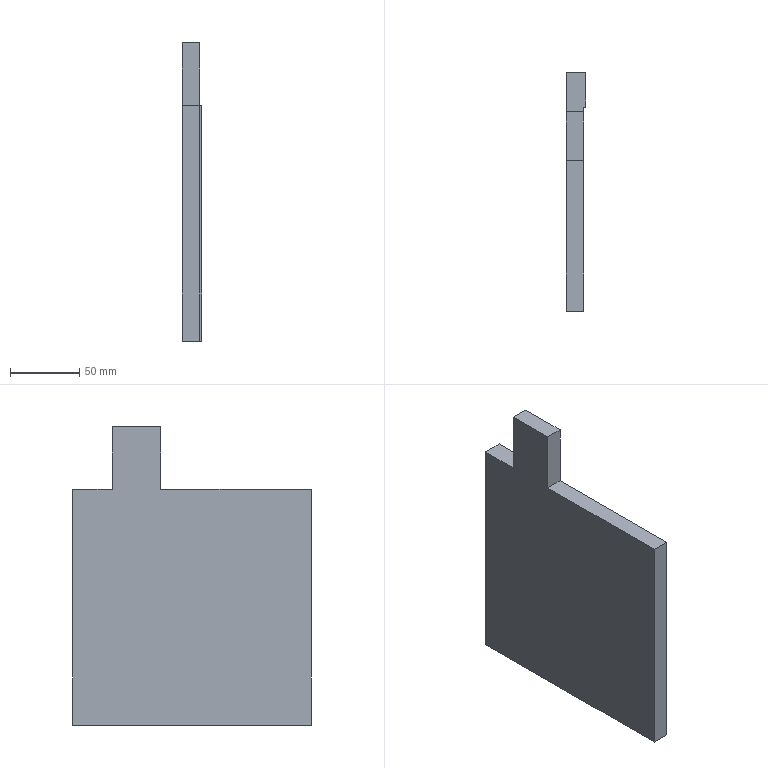Part | SolidWorks | features ICE 2, 3DProfileFeature 1, Extrusion 1, HoleWzd 1 | 1 solid | 12 faces | box 14 x 172 x 215 mm | volume 391562 mm3 | plane 12
STEP:
#1=CARTESIAN_POINT('',(12.5,0.,85.));
#2=VERTEX_POINT('',#1);
#3=CARTESIAN_POINT('',(12.5,108.5,85.));
#4=VERTEX_POINT('',#3);
#5=CARTESIAN_POINT('',(12.5,147.,85.));
#6=DIRECTION('',(0.,1.,0.));
#7=VECTOR('',#6,1000.);
#8=LINE('',#5,#7);
#9=EDGE_CURVE('',#2,#4,#8,.T.);
#10=ORIENTED_EDGE('',*,*,#9,.T.);
#11=CARTESIAN_POINT('',(0.,108.5,85.));
#12=VERTEX_POINT('',#11);
#13=CARTESIAN_POINT('',(12.5,108.5,85.));
#14=DIRECTION('',(-1.,0.,0.));
#15=VECTOR('',#14,1000.);
#16=LINE('',#13,#15);
#17=EDGE_CURVE('',#4,#12,#16,.T.);
#18=ORIENTED_EDGE('',*,*,#17,.T.);
#19=CARTESIAN_POINT('',(0.,0.,85.));
#20=VERTEX_POINT('',#19);
#21=CARTESIAN_POINT('',(0.,0.,85.));
#22=DIRECTION('',(0.,-1.,0.));
#23=VECTOR('',#22,1000.);
#24=LINE('',#21,#23);
#25=EDGE_CURVE('',#12,#20,#24,.T.);
#26=ORIENTED_EDGE('',*,*,#25,.T.);
#27=CARTESIAN_POINT('',(12.5,0.,85.));
#28=DIRECTION('',(1.,0.,0.));
#29=VECTOR('',#28,1000.);
#30=LINE('',#27,#29);
#31=EDGE_CURVE('',#20,#2,#30,.T.);
#32=ORIENTED_EDGE('',*,*,#31,.T.);
#33=EDGE_LOOP('',(#10,#18,#26,#32));
#34=FACE_OUTER_BOUND('',#33,.T.);
#35=CARTESIAN_POINT('',(0.,0.,85.));
#36=DIRECTION('',(0.,0.,-1.));
#37=DIRECTION('',(-1.,0.,0.));
#38=AXIS2_PLACEMENT_3D('',#35,#36,#37);
#39=PLANE('',#38);
#40=ADVANCED_FACE('',(#34),#39,.F.);
#41=CARTESIAN_POINT('',(0.,0.,-85.));
#42=VERTEX_POINT('',#41);
#43=CARTESIAN_POINT('',(12.5,0.,-85.));
#44=VERTEX_POINT('',#43);
#45=CARTESIAN_POINT('',(12.5,0.,-85.));
#46=DIRECTION('',(1.,0.,0.));
#47=VECTOR('',#46,1000.);
#48=LINE('',#45,#47);
#49=EDGE_CURVE('',#42,#44,#48,.T.);
#50=ORIENTED_EDGE('',*,*,#49,.T.);
#51=CARTESIAN_POINT('',(12.5,0.,85.));
#52=DIRECTION('',(0.,0.,-1.));
#53=VECTOR('',#52,1000.);
#54=LINE('',#51,#53);
#55=EDGE_CURVE('',#2,#44,#54,.T.);
#56=ORIENTED_EDGE('',*,*,#55,.F.);
#57=ORIENTED_EDGE('',*,*,#31,.F.);
#58=CARTESIAN_POINT('',(0.,0.,85.));
#59=DIRECTION('',(0.,0.,-1.));
#60=VECTOR('',#59,1000.);
#61=LINE('',#58,#60);
#62=EDGE_CURVE('',#20,#42,#61,.T.);
#63=ORIENTED_EDGE('',*,*,#62,.T.);
#64=EDGE_LOOP('',(#50,#56,#57,#63));
#65=FACE_OUTER_BOUND('',#64,.T.);
#66=CARTESIAN_POINT('',(12.5,0.,85.));
#67=DIRECTION('',(0.,1.,0.));
#68=DIRECTION('',(-1.,0.,0.));
#69=AXIS2_PLACEMENT_3D('',#66,#67,#68);
#70=PLANE('',#69);
#71=ADVANCED_FACE('',(#65),#70,.F.);
#72=CARTESIAN_POINT('',(12.5,147.,-85.));
#73=VERTEX_POINT('',#72);
#74=CARTESIAN_POINT('',(12.5,147.,-85.));
#75=DIRECTION('',(0.,1.,0.));
#76=VECTOR('',#75,1000.);
#77=LINE('',#74,#76);
#78=EDGE_CURVE('',#44,#73,#77,.T.);
#79=ORIENTED_EDGE('',*,*,#78,.T.);
#80=CARTESIAN_POINT('',(12.5,147.,85.));
#81=VERTEX_POINT('',#80);
#82=CARTESIAN_POINT('',(12.5,147.,85.));
#83=DIRECTION('',(0.,0.,-1.));
#84=VECTOR('',#83,1000.);
#85=LINE('',#82,#84);
#86=EDGE_CURVE('',#81,#73,#85,.T.);
#87=ORIENTED_EDGE('',*,*,#86,.F.);
#88=CARTESIAN_POINT('',(12.5,143.5,85.));
#89=VERTEX_POINT('',#88);
#90=CARTESIAN_POINT('',(12.5,147.,85.));
#91=DIRECTION('',(0.,1.,0.));
#92=VECTOR('',#91,1000.);
#93=LINE('',#90,#92);
#94=EDGE_CURVE('',#89,#81,#93,.T.);
#95=ORIENTED_EDGE('',*,*,#94,.F.);
#96=CARTESIAN_POINT('',(12.5,143.5,130.));
#97=VERTEX_POINT('',#96);
#98=CARTESIAN_POINT('',(12.5,143.5,130.));
#99=DIRECTION('',(0.,0.,-1.));
#100=VECTOR('',#99,1000.);
#101=LINE('',#98,#100);
#102=EDGE_CURVE('',#97,#89,#101,.T.);
#103=ORIENTED_EDGE('',*,*,#102,.F.);
#104=CARTESIAN_POINT('',(12.5,108.5,130.));
#105=VERTEX_POINT('',#104);
#106=CARTESIAN_POINT('',(12.5,143.5,130.));
#107=DIRECTION('',(0.,-1.,0.));
#108=VECTOR('',#107,1000.);
#109=LINE('',#106,#108);
#110=EDGE_CURVE('',#97,#105,#109,.T.);
#111=ORIENTED_EDGE('',*,*,#110,.T.);
#112=CARTESIAN_POINT('',(12.5,108.5,130.));
#113=DIRECTION('',(0.,0.,-1.));
#114=VECTOR('',#113,1000.);
#115=LINE('',#112,#114);
#116=EDGE_CURVE('',#105,#4,#115,.T.);
#117=ORIENTED_EDGE('',*,*,#116,.T.);
#118=ORIENTED_EDGE('',*,*,#9,.F.);
#119=ORIENTED_EDGE('',*,*,#55,.T.);
#120=EDGE_LOOP('',(#79,#87,#95,#103,#111,#117,#118,#119));
#121=FACE_OUTER_BOUND('',#120,.T.);
#122=CARTESIAN_POINT('',(12.5,147.,85.));
#123=DIRECTION('',(-1.,0.,0.));
#124=DIRECTION('',(0.,-1.,0.));
#125=AXIS2_PLACEMENT_3D('',#122,#123,#124);
#126=PLANE('',#125);
#127=ADVANCED_FACE('',(#121),#126,.F.);
#128=CARTESIAN_POINT('',(14.,147.,-85.));
#129=VERTEX_POINT('',#128);
#130=CARTESIAN_POINT('',(14.,147.,-85.));
#131=DIRECTION('',(1.,0.,0.));
#132=VECTOR('',#131,1000.);
#133=LINE('',#130,#132);
#134=EDGE_CURVE('',#73,#129,#133,.T.);
#135=ORIENTED_EDGE('',*,*,#134,.T.);
#136=CARTESIAN_POINT('',(14.,147.,85.));
#137=VERTEX_POINT('',#136);
#138=CARTESIAN_POINT('',(14.,147.,85.));
#139=DIRECTION('',(0.,0.,-1.));
#140=VECTOR('',#139,1000.);
#141=LINE('',#138,#140);
#142=EDGE_CURVE('',#137,#129,#141,.T.);
#143=ORIENTED_EDGE('',*,*,#142,.F.);
#144=CARTESIAN_POINT('',(14.,147.,85.));
#145=DIRECTION('',(1.,0.,0.));
#146=VECTOR('',#145,1000.);
#147=LINE('',#144,#146);
#148=EDGE_CURVE('',#81,#137,#147,.T.);
#149=ORIENTED_EDGE('',*,*,#148,.F.);
#150=ORIENTED_EDGE('',*,*,#86,.T.);
#151=EDGE_LOOP('',(#135,#143,#149,#150));
#152=FACE_OUTER_BOUND('',#151,.T.);
#153=CARTESIAN_POINT('',(14.,147.,85.));
#154=DIRECTION('',(0.,1.,0.));
#155=DIRECTION('',(0.,0.,1.));
#156=AXIS2_PLACEMENT_3D('',#153,#154,#155);
#157=PLANE('',#156);
#158=ADVANCED_FACE('',(#152),#157,.F.);
#159=CARTESIAN_POINT('',(14.,172.,-85.));
#160=VERTEX_POINT('',#159);
#161=CARTESIAN_POINT('',(14.,172.,-85.));
#162=DIRECTION('',(0.,1.,0.));
#163=VECTOR('',#162,1000.);
#164=LINE('',#161,#163);
#165=EDGE_CURVE('',#129,#160,#164,.T.);
#166=ORIENTED_EDGE('',*,*,#165,.T.);
#167=CARTESIAN_POINT('',(14.,172.,85.));
#168=VERTEX_POINT('',#167);
#169=CARTESIAN_POINT('',(14.,172.,85.));
#170=DIRECTION('',(0.,0.,-1.));
#171=VECTOR('',#170,1000.);
#172=LINE('',#169,#171);
#173=EDGE_CURVE('',#168,#160,#172,.T.);
#174=ORIENTED_EDGE('',*,*,#173,.F.);
#175=CARTESIAN_POINT('',(14.,172.,85.));
#176=DIRECTION('',(0.,1.,0.));
#177=VECTOR('',#176,1000.);
#178=LINE('',#175,#177);
#179=EDGE_CURVE('',#137,#168,#178,.T.);
#180=ORIENTED_EDGE('',*,*,#179,.F.);
#181=ORIENTED_EDGE('',*,*,#142,.T.);
#182=EDGE_LOOP('',(#166,#174,#180,#181));
#183=FACE_OUTER_BOUND('',#182,.T.);
#184=CARTESIAN_POINT('',(14.,172.,85.));
#185=DIRECTION('',(-1.,0.,0.));
#186=DIRECTION('',(0.,-1.,0.));
#187=AXIS2_PLACEMENT_3D('',#184,#185,#186);
#188=PLANE('',#187);
#189=ADVANCED_FACE('',(#183),#188,.F.);
#190=CARTESIAN_POINT('',(0.,172.,-85.));
#191=VERTEX_POINT('',#190);
#192=CARTESIAN_POINT('',(0.,172.,-85.));
#193=DIRECTION('',(-1.,0.,0.));
#194=VECTOR('',#193,1000.);
#195=LINE('',#192,#194);
#196=EDGE_CURVE('',#160,#191,#195,.T.);
#197=ORIENTED_EDGE('',*,*,#196,.T.);
#198=CARTESIAN_POINT('',(0.,172.,85.));
#199=VERTEX_POINT('',#198);
#200=CARTESIAN_POINT('',(0.,172.,85.));
#201=DIRECTION('',(0.,0.,-1.));
#202=VECTOR('',#201,1000.);
#203=LINE('',#200,#202);
#204=EDGE_CURVE('',#199,#191,#203,.T.);
#205=ORIENTED_EDGE('',*,*,#204,.F.);
#206=CARTESIAN_POINT('',(0.,172.,85.));
#207=DIRECTION('',(-1.,0.,0.));
#208=VECTOR('',#207,1000.);
#209=LINE('',#206,#208);
#210=EDGE_CURVE('',#168,#199,#209,.T.);
#211=ORIENTED_EDGE('',*,*,#210,.F.);
#212=ORIENTED_EDGE('',*,*,#173,.T.);
#213=EDGE_LOOP('',(#197,#205,#211,#212));
#214=FACE_OUTER_BOUND('',#213,.T.);
#215=CARTESIAN_POINT('',(0.,172.,85.));
#216=DIRECTION('',(0.,-1.,0.));
#217=DIRECTION('',(0.,0.,-1.));
#218=AXIS2_PLACEMENT_3D('',#215,#216,#217);
#219=PLANE('',#218);
#220=ADVANCED_FACE('',(#214),#219,.F.);
#221=CARTESIAN_POINT('',(0.,0.,-85.));
#222=DIRECTION('',(0.,-1.,0.));
#223=VECTOR('',#222,1000.);
#224=LINE('',#221,#223);
#225=EDGE_CURVE('',#191,#42,#224,.T.);
#226=ORIENTED_EDGE('',*,*,#225,.T.);
#227=ORIENTED_EDGE('',*,*,#62,.F.);
#228=ORIENTED_EDGE('',*,*,#25,.F.);
#229=CARTESIAN_POINT('',(0.,108.5,130.));
#230=VERTEX_POINT('',#229);
#231=CARTESIAN_POINT('',(0.,108.5,130.));
#232=DIRECTION('',(0.,0.,-1.));
#233=VECTOR('',#232,1000.);
#234=LINE('',#231,#233);
#235=EDGE_CURVE('',#230,#12,#234,.T.);
#236=ORIENTED_EDGE('',*,*,#235,.F.);
#237=CARTESIAN_POINT('',(0.,143.5,130.));
#238=VERTEX_POINT('',#237);
#239=CARTESIAN_POINT('',(0.,143.5,130.));
#240=DIRECTION('',(0.,1.,0.));
#241=VECTOR('',#240,1000.);
#242=LINE('',#239,#241);
#243=EDGE_CURVE('',#230,#238,#242,.T.);
#244=ORIENTED_EDGE('',*,*,#243,.T.);
#245=CARTESIAN_POINT('',(0.,143.5,85.));
#246=VERTEX_POINT('',#245);
#247=CARTESIAN_POINT('',(0.,143.5,130.));
#248=DIRECTION('',(0.,0.,-1.));
#249=VECTOR('',#248,1000.);
#250=LINE('',#247,#249);
#251=EDGE_CURVE('',#238,#246,#250,.T.);
#252=ORIENTED_EDGE('',*,*,#251,.T.);
#253=CARTESIAN_POINT('',(0.,0.,85.));
#254=DIRECTION('',(0.,-1.,0.));
#255=VECTOR('',#254,1000.);
#256=LINE('',#253,#255);
#257=EDGE_CURVE('',#199,#246,#256,.T.);
#258=ORIENTED_EDGE('',*,*,#257,.F.);
#259=ORIENTED_EDGE('',*,*,#204,.T.);
#260=EDGE_LOOP('',(#226,#227,#228,#236,#244,#252,#258,#259));
#261=FACE_OUTER_BOUND('',#260,.T.);
#262=CARTESIAN_POINT('',(0.,0.,85.));
#263=DIRECTION('',(1.,0.,0.));
#264=DIRECTION('',(0.,1.,0.));
#265=AXIS2_PLACEMENT_3D('',#262,#263,#264);
#266=PLANE('',#265);
#267=ADVANCED_FACE('',(#261),#266,.F.);
#268=ORIENTED_EDGE('',*,*,#257,.T.);
#269=CARTESIAN_POINT('',(12.5,143.5,85.));
#270=DIRECTION('',(1.,0.,0.));
#271=VECTOR('',#270,1000.);
#272=LINE('',#269,#271);
#273=EDGE_CURVE('',#246,#89,#272,.T.);
#274=ORIENTED_EDGE('',*,*,#273,.T.);
#275=ORIENTED_EDGE('',*,*,#94,.T.);
#276=ORIENTED_EDGE('',*,*,#148,.T.);
#277=ORIENTED_EDGE('',*,*,#179,.T.);
#278=ORIENTED_EDGE('',*,*,#210,.T.);
#279=EDGE_LOOP('',(#268,#274,#275,#276,#277,#278));
#280=FACE_OUTER_BOUND('',#279,.T.);
#281=CARTESIAN_POINT('',(0.,0.,85.));
#282=DIRECTION('',(0.,0.,-1.));
#283=DIRECTION('',(-1.,0.,0.));
#284=AXIS2_PLACEMENT_3D('',#281,#282,#283);
#285=PLANE('',#284);
#286=ADVANCED_FACE('',(#280),#285,.F.);
#287=ORIENTED_EDGE('',*,*,#49,.F.);
#288=ORIENTED_EDGE('',*,*,#225,.F.);
#289=ORIENTED_EDGE('',*,*,#196,.F.);
#290=ORIENTED_EDGE('',*,*,#165,.F.);
#291=ORIENTED_EDGE('',*,*,#134,.F.);
#292=ORIENTED_EDGE('',*,*,#78,.F.);
#293=EDGE_LOOP('',(#287,#288,#289,#290,#291,#292));
#294=FACE_OUTER_BOUND('',#293,.T.);
#295=CARTESIAN_POINT('',(0.,0.,-85.));
#296=DIRECTION('',(0.,0.,-1.));
#297=DIRECTION('',(-1.,0.,0.));
#298=AXIS2_PLACEMENT_3D('',#295,#296,#297);
#299=PLANE('',#298);
#300=ADVANCED_FACE('',(#294),#299,.T.);
#301=ORIENTED_EDGE('',*,*,#273,.F.);
#302=ORIENTED_EDGE('',*,*,#251,.F.);
#303=CARTESIAN_POINT('',(12.5,143.5,130.));
#304=DIRECTION('',(1.,0.,0.));
#305=VECTOR('',#304,1000.);
#306=LINE('',#303,#305);
#307=EDGE_CURVE('',#238,#97,#306,.T.);
#308=ORIENTED_EDGE('',*,*,#307,.T.);
#309=ORIENTED_EDGE('',*,*,#102,.T.);
#310=EDGE_LOOP('',(#301,#302,#308,#309));
#311=FACE_OUTER_BOUND('',#310,.T.);
#312=CARTESIAN_POINT('',(12.5,143.5,130.));
#313=DIRECTION('',(0.,1.,0.));
#314=DIRECTION('',(0.,0.,1.));
#315=AXIS2_PLACEMENT_3D('',#312,#313,#314);
#316=PLANE('',#315);
#317=ADVANCED_FACE('',(#311),#316,.T.);
#318=ORIENTED_EDGE('',*,*,#17,.F.);
#319=ORIENTED_EDGE('',*,*,#116,.F.);
#320=CARTESIAN_POINT('',(12.5,108.5,130.));
#321=DIRECTION('',(-1.,0.,0.));
#322=VECTOR('',#321,1000.);
#323=LINE('',#320,#322);
#324=EDGE_CURVE('',#105,#230,#323,.T.);
#325=ORIENTED_EDGE('',*,*,#324,.T.);
#326=ORIENTED_EDGE('',*,*,#235,.T.);
#327=EDGE_LOOP('',(#318,#319,#325,#326));
#328=FACE_OUTER_BOUND('',#327,.T.);
#329=CARTESIAN_POINT('',(12.5,108.5,130.));
#330=DIRECTION('',(0.,-1.,0.));
#331=DIRECTION('',(0.,0.,-1.));
#332=AXIS2_PLACEMENT_3D('',#329,#330,#331);
#333=PLANE('',#332);
#334=ADVANCED_FACE('',(#328),#333,.T.);
#335=ORIENTED_EDGE('',*,*,#110,.F.);
#336=ORIENTED_EDGE('',*,*,#307,.F.);
#337=ORIENTED_EDGE('',*,*,#243,.F.);
#338=ORIENTED_EDGE('',*,*,#324,.F.);
#339=EDGE_LOOP('',(#335,#336,#337,#338));
#340=FACE_OUTER_BOUND('',#339,.T.);
#341=CARTESIAN_POINT('',(0.,0.,130.));
#342=DIRECTION('',(0.,0.,-1.));
#343=DIRECTION('',(-1.,0.,0.));
#344=AXIS2_PLACEMENT_3D('',#341,#342,#343);
#345=PLANE('',#344);
#346=ADVANCED_FACE('',(#340),#345,.F.);
#347=CLOSED_SHELL('',(#40,#71,#127,#158,#189,#220,#267,#286,#300,#317,#334,#346));
#348=MANIFOLD_SOLID_BREP('',#347);
#349=CARTESIAN_POINT('',(0.,0.,0.));
#350=DIRECTION('',(0.,0.,1.));
#351=DIRECTION('',(1.,0.,0.));
#352=AXIS2_PLACEMENT_3D('',#349,#350,#351);
#353=(LENGTH_UNIT()NAMED_UNIT(*)SI_UNIT(.MILLI.,.METRE.));
#354=UNCERTAINTY_MEASURE_WITH_UNIT(LENGTH_MEASURE(0.00001),#353,'','');
#355=(NAMED_UNIT(*)PLANE_ANGLE_UNIT()SI_UNIT($,.RADIAN.));
#356=(NAMED_UNIT(*)SI_UNIT($,.STERADIAN.)SOLID_ANGLE_UNIT());
#357=(GEOMETRIC_REPRESENTATION_CONTEXT(3)GLOBAL_UNCERTAINTY_ASSIGNED_CONTEXT((#354))GLOBAL_UNIT_ASSIGNED_CONTEXT((#353,#355,#356))REPRESENTATION_CONTEXT('',''));
#358=ADVANCED_BREP_SHAPE_REPRESENTATION('',(#348,#352),#357);